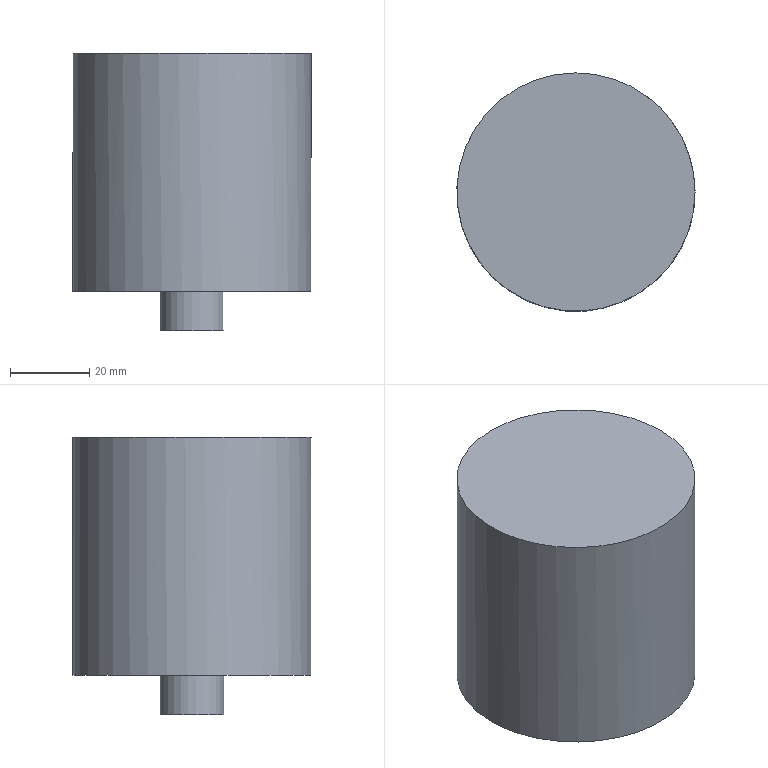Part | NX | features solid 2 | 1 solid | 5 faces | box 60 x 60 x 70 mm | volume 171657 mm3 | plane 3 | cylinder 2 | commonest cylinder face diameters 16 x1 60 x1
STEP:
#1=CARTESIAN_POINT('',(-1295.,-290.,45.));
#2=VERTEX_POINT('',#1);
#3=CARTESIAN_POINT('',(-1325.,-290.,45.));
#4=DIRECTION('',(0.,0.,1.));
#5=DIRECTION('',(1.,0.,0.));
#6=AXIS2_PLACEMENT_3D('',#3,#4,#5);
#7=CIRCLE('',#6,30.);
#8=EDGE_CURVE('',#2,#2,#7,.T.);
#9=ORIENTED_EDGE('',*,*,#8,.T.);
#10=EDGE_LOOP('',(#9));
#11=FACE_BOUND('',#10,.T.);
#12=CARTESIAN_POINT('',(-1325.,-290.,45.));
#13=DIRECTION('',(0.,0.,1.));
#14=DIRECTION('',(-1.,0.,0.));
#15=AXIS2_PLACEMENT_3D('',#12,#13,#14);
#16=PLANE('',#15);
#17=ADVANCED_FACE('',(#11),#16,.T.);
#18=CARTESIAN_POINT('',(-1325.,-282.,-15.));
#19=VERTEX_POINT('',#18);
#20=CARTESIAN_POINT('',(-1325.,-290.,-15.));
#21=DIRECTION('',(0.,0.,1.));
#22=DIRECTION('',(0.,1.,0.));
#23=AXIS2_PLACEMENT_3D('',#20,#21,#22);
#24=CIRCLE('',#23,8.);
#25=EDGE_CURVE('',#19,#19,#24,.T.);
#26=ORIENTED_EDGE('',*,*,#25,.T.);
#27=EDGE_LOOP('',(#26));
#28=FACE_BOUND('',#27,.T.);
#29=CARTESIAN_POINT('',(-1325.,-260.,-15.));
#30=VERTEX_POINT('',#29);
#31=CARTESIAN_POINT('',(-1325.,-290.,-15.));
#32=DIRECTION('',(0.,0.,-1.));
#33=DIRECTION('',(0.,1.,0.));
#34=AXIS2_PLACEMENT_3D('',#31,#32,#33);
#35=CIRCLE('',#34,30.);
#36=EDGE_CURVE('',#30,#30,#35,.T.);
#37=ORIENTED_EDGE('',*,*,#36,.T.);
#38=EDGE_LOOP('',(#37));
#39=FACE_BOUND('',#38,.T.);
#40=CARTESIAN_POINT('',(-1325.,-290.,-15.));
#41=DIRECTION('',(0.,0.,-1.));
#42=DIRECTION('',(1.,0.,0.));
#43=AXIS2_PLACEMENT_3D('',#40,#41,#42);
#44=PLANE('',#43);
#45=ADVANCED_FACE('',(#28,#39),#44,.T.);
#46=ORIENTED_EDGE('',*,*,#8,.F.);
#47=EDGE_LOOP('',(#46));
#48=FACE_BOUND('',#47,.T.);
#49=ORIENTED_EDGE('',*,*,#36,.F.);
#50=EDGE_LOOP('',(#49));
#51=FACE_BOUND('',#50,.T.);
#52=CARTESIAN_POINT('',(-1325.,-290.,-5.));
#53=DIRECTION('',(0.,0.,1.));
#54=DIRECTION('',(-1.,0.,0.));
#55=AXIS2_PLACEMENT_3D('',#52,#53,#54);
#56=CYLINDRICAL_SURFACE('',#55,30.);
#57=ADVANCED_FACE('',(#48,#51),#56,.T.);
#58=CARTESIAN_POINT('',(-1325.,-282.,-25.));
#59=VERTEX_POINT('',#58);
#60=CARTESIAN_POINT('',(-1325.,-290.,-25.));
#61=DIRECTION('',(0.,0.,1.));
#62=DIRECTION('',(0.,1.,0.));
#63=AXIS2_PLACEMENT_3D('',#60,#61,#62);
#64=CIRCLE('',#63,8.);
#65=EDGE_CURVE('',#59,#59,#64,.F.);
#66=ORIENTED_EDGE('',*,*,#65,.T.);
#67=EDGE_LOOP('',(#66));
#68=FACE_BOUND('',#67,.T.);
#69=CARTESIAN_POINT('',(-1325.,-290.,-25.));
#70=DIRECTION('',(0.,0.,-1.));
#71=DIRECTION('',(1.,0.,0.));
#72=AXIS2_PLACEMENT_3D('',#69,#70,#71);
#73=PLANE('',#72);
#74=ADVANCED_FACE('',(#68),#73,.T.);
#75=ORIENTED_EDGE('',*,*,#65,.F.);
#76=EDGE_LOOP('',(#75));
#77=FACE_BOUND('',#76,.T.);
#78=ORIENTED_EDGE('',*,*,#25,.F.);
#79=EDGE_LOOP('',(#78));
#80=FACE_BOUND('',#79,.T.);
#81=CARTESIAN_POINT('',(-1325.,-290.,-5.));
#82=DIRECTION('',(0.,0.,-1.));
#83=DIRECTION('',(1.,0.,0.));
#84=AXIS2_PLACEMENT_3D('',#81,#82,#83);
#85=CYLINDRICAL_SURFACE('',#84,8.);
#86=ADVANCED_FACE('',(#77,#80),#85,.T.);
#87=CLOSED_SHELL('',(#17,#45,#57,#74,#86));
#88=MANIFOLD_SOLID_BREP('',#87);
#89=(LENGTH_UNIT()NAMED_UNIT(*)SI_UNIT(.MILLI.,.METRE.));
#90=UNCERTAINTY_MEASURE_WITH_UNIT(LENGTH_MEASURE(0.00001),#89,'','');
#91=(NAMED_UNIT(*)PLANE_ANGLE_UNIT()SI_UNIT($,.RADIAN.));
#92=(NAMED_UNIT(*)SI_UNIT($,.STERADIAN.)SOLID_ANGLE_UNIT());
#93=(GEOMETRIC_REPRESENTATION_CONTEXT(3)GLOBAL_UNCERTAINTY_ASSIGNED_CONTEXT((#90))GLOBAL_UNIT_ASSIGNED_CONTEXT((#89,#91,#92))REPRESENTATION_CONTEXT('',''));
#94=ADVANCED_BREP_SHAPE_REPRESENTATION('',(#88),#93);